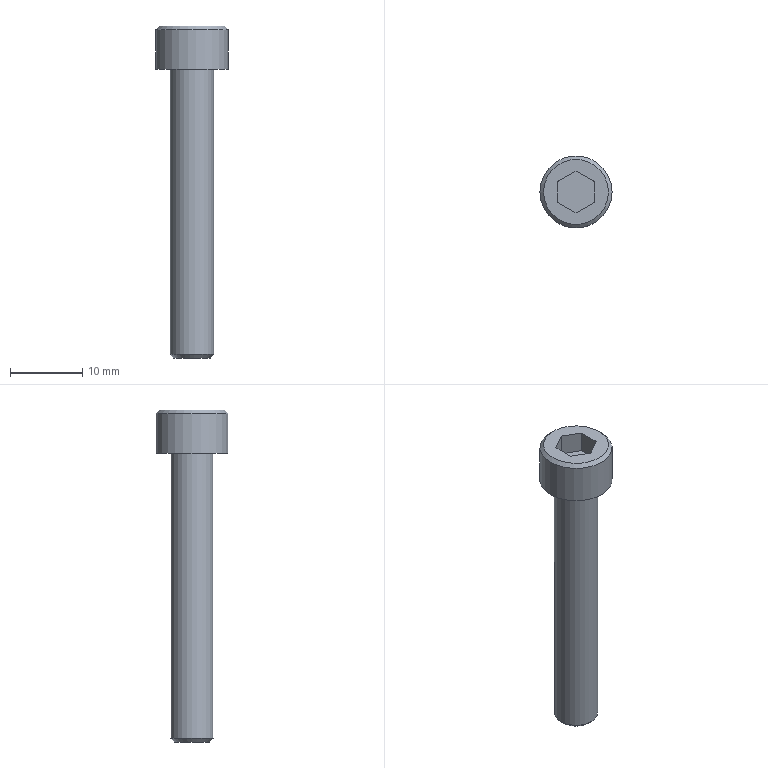Part | NX | features M6.00-50.00 2 | 1 solid | 14 faces | box 10 x 10 x 46 mm | volume 1531 mm3 | plane 10 | cylinder 2 | cone 2 | commonest cylinder face diameters 6 x1 10 x1
STEP:
#1=CARTESIAN_POINT('',(-39.5,190.75,-1.5));
#2=VERTEX_POINT('',#1);
#3=CARTESIAN_POINT('',(-44.,190.75,-1.5));
#4=DIRECTION('',(0.,0.,1.));
#5=DIRECTION('',(1.,0.,0.));
#6=AXIS2_PLACEMENT_3D('',#3,#4,#5);
#7=CIRCLE('',#6,4.5);
#8=EDGE_CURVE('',#2,#2,#7,.T.);
#9=ORIENTED_EDGE('',*,*,#8,.T.);
#10=EDGE_LOOP('',(#9));
#11=FACE_BOUND('',#10,.T.);
#12=CARTESIAN_POINT('',(-46.5,192.193,-1.5));
#13=VERTEX_POINT('',#12);
#14=CARTESIAN_POINT('',(-46.5,189.307,-1.5));
#15=VERTEX_POINT('',#14);
#16=CARTESIAN_POINT('',(-46.5,192.193,-1.5));
#17=DIRECTION('',(0.,-1.,0.));
#18=VECTOR('',#17,1000.);
#19=LINE('',#16,#18);
#20=EDGE_CURVE('',#13,#15,#19,.T.);
#21=ORIENTED_EDGE('',*,*,#20,.F.);
#22=CARTESIAN_POINT('',(-44.,193.637,-1.5));
#23=VERTEX_POINT('',#22);
#24=CARTESIAN_POINT('',(-44.,193.637,-1.5));
#25=DIRECTION('',(-0.866,-0.5,0.));
#26=VECTOR('',#25,1000.);
#27=LINE('',#24,#26);
#28=EDGE_CURVE('',#23,#13,#27,.T.);
#29=ORIENTED_EDGE('',*,*,#28,.F.);
#30=CARTESIAN_POINT('',(-41.5,192.193,-1.5));
#31=VERTEX_POINT('',#30);
#32=CARTESIAN_POINT('',(-41.5,192.193,-1.5));
#33=DIRECTION('',(-0.866,0.5,0.));
#34=VECTOR('',#33,1000.);
#35=LINE('',#32,#34);
#36=EDGE_CURVE('',#31,#23,#35,.T.);
#37=ORIENTED_EDGE('',*,*,#36,.F.);
#38=CARTESIAN_POINT('',(-41.5,189.307,-1.5));
#39=VERTEX_POINT('',#38);
#40=CARTESIAN_POINT('',(-41.5,189.307,-1.5));
#41=DIRECTION('',(0.,1.,0.));
#42=VECTOR('',#41,1000.);
#43=LINE('',#40,#42);
#44=EDGE_CURVE('',#39,#31,#43,.T.);
#45=ORIENTED_EDGE('',*,*,#44,.F.);
#46=CARTESIAN_POINT('',(-44.,187.863,-1.5));
#47=VERTEX_POINT('',#46);
#48=CARTESIAN_POINT('',(-44.,187.863,-1.5));
#49=DIRECTION('',(0.866,0.5,0.));
#50=VECTOR('',#49,1000.);
#51=LINE('',#48,#50);
#52=EDGE_CURVE('',#47,#39,#51,.T.);
#53=ORIENTED_EDGE('',*,*,#52,.F.);
#54=CARTESIAN_POINT('',(-46.5,189.307,-1.5));
#55=DIRECTION('',(0.866,-0.5,0.));
#56=VECTOR('',#55,1000.);
#57=LINE('',#54,#56);
#58=EDGE_CURVE('',#15,#47,#57,.T.);
#59=ORIENTED_EDGE('',*,*,#58,.F.);
#60=EDGE_LOOP('',(#21,#29,#37,#45,#53,#59));
#61=FACE_BOUND('',#60,.T.);
#62=CARTESIAN_POINT('',(-44.,190.75,-1.5));
#63=DIRECTION('',(0.,0.,1.));
#64=DIRECTION('',(1.,0.,0.));
#65=AXIS2_PLACEMENT_3D('',#62,#63,#64);
#66=PLANE('',#65);
#67=ADVANCED_FACE('',(#11,#61),#66,.T.);
#68=CARTESIAN_POINT('',(-41.,190.75,-7.5));
#69=VERTEX_POINT('',#68);
#70=CARTESIAN_POINT('',(-44.,190.75,-7.5));
#71=DIRECTION('',(0.,0.,-1.));
#72=DIRECTION('',(1.,0.,0.));
#73=AXIS2_PLACEMENT_3D('',#70,#71,#72);
#74=CIRCLE('',#73,3.);
#75=EDGE_CURVE('',#69,#69,#74,.T.);
#76=ORIENTED_EDGE('',*,*,#75,.F.);
#77=EDGE_LOOP('',(#76));
#78=FACE_BOUND('',#77,.T.);
#79=CARTESIAN_POINT('',(-39.,190.75,-7.5));
#80=VERTEX_POINT('',#79);
#81=CARTESIAN_POINT('',(-44.,190.75,-7.5));
#82=DIRECTION('',(0.,0.,1.));
#83=DIRECTION('',(1.,0.,0.));
#84=AXIS2_PLACEMENT_3D('',#81,#82,#83);
#85=CIRCLE('',#84,5.);
#86=EDGE_CURVE('',#80,#80,#85,.T.);
#87=ORIENTED_EDGE('',*,*,#86,.F.);
#88=EDGE_LOOP('',(#87));
#89=FACE_BOUND('',#88,.T.);
#90=CARTESIAN_POINT('',(-44.,190.75,-7.5));
#91=DIRECTION('',(0.,0.,-1.));
#92=DIRECTION('',(-1.,0.,0.));
#93=AXIS2_PLACEMENT_3D('',#90,#91,#92);
#94=PLANE('',#93);
#95=ADVANCED_FACE('',(#78,#89),#94,.T.);
#96=CARTESIAN_POINT('',(-39.,190.75,-2.));
#97=VERTEX_POINT('',#96);
#98=CARTESIAN_POINT('',(-44.,190.75,-2.));
#99=DIRECTION('',(0.,0.,1.));
#100=DIRECTION('',(1.,0.,0.));
#101=AXIS2_PLACEMENT_3D('',#98,#99,#100);
#102=CIRCLE('',#101,5.);
#103=EDGE_CURVE('',#97,#97,#102,.F.);
#104=ORIENTED_EDGE('',*,*,#103,.T.);
#105=EDGE_LOOP('',(#104));
#106=FACE_BOUND('',#105,.T.);
#107=ORIENTED_EDGE('',*,*,#86,.T.);
#108=EDGE_LOOP('',(#107));
#109=FACE_BOUND('',#108,.T.);
#110=CARTESIAN_POINT('',(-44.,190.75,-7.5));
#111=DIRECTION('',(0.,0.,1.));
#112=DIRECTION('',(1.,0.,0.));
#113=AXIS2_PLACEMENT_3D('',#110,#111,#112);
#114=CYLINDRICAL_SURFACE('',#113,5.);
#115=ADVANCED_FACE('',(#106,#109),#114,.T.);
#116=CARTESIAN_POINT('',(-46.5,190.75,-47.5));
#117=VERTEX_POINT('',#116);
#118=CARTESIAN_POINT('',(-44.,190.75,-47.5));
#119=DIRECTION('',(0.,0.,-1.));
#120=DIRECTION('',(-1.,0.,0.));
#121=AXIS2_PLACEMENT_3D('',#118,#119,#120);
#122=CIRCLE('',#121,2.5);
#123=EDGE_CURVE('',#117,#117,#122,.T.);
#124=ORIENTED_EDGE('',*,*,#123,.T.);
#125=EDGE_LOOP('',(#124));
#126=FACE_BOUND('',#125,.T.);
#127=CARTESIAN_POINT('',(-44.,190.75,-47.5));
#128=DIRECTION('',(0.,0.,-1.));
#129=DIRECTION('',(-1.,0.,0.));
#130=AXIS2_PLACEMENT_3D('',#127,#128,#129);
#131=PLANE('',#130);
#132=ADVANCED_FACE('',(#126),#131,.T.);
#133=CARTESIAN_POINT('',(-47.,190.75,-47.));
#134=VERTEX_POINT('',#133);
#135=CARTESIAN_POINT('',(-44.,190.75,-47.));
#136=DIRECTION('',(0.,0.,-1.));
#137=DIRECTION('',(-1.,0.,0.));
#138=AXIS2_PLACEMENT_3D('',#135,#136,#137);
#139=CIRCLE('',#138,3.);
#140=EDGE_CURVE('',#134,#134,#139,.F.);
#141=ORIENTED_EDGE('',*,*,#140,.T.);
#142=EDGE_LOOP('',(#141));
#143=FACE_BOUND('',#142,.T.);
#144=ORIENTED_EDGE('',*,*,#75,.T.);
#145=EDGE_LOOP('',(#144));
#146=FACE_BOUND('',#145,.T.);
#147=CARTESIAN_POINT('',(-44.,190.75,-7.5));
#148=DIRECTION('',(0.,0.,-1.));
#149=DIRECTION('',(1.,0.,0.));
#150=AXIS2_PLACEMENT_3D('',#147,#148,#149);
#151=CYLINDRICAL_SURFACE('',#150,3.);
#152=ADVANCED_FACE('',(#143,#146),#151,.T.);
#153=ORIENTED_EDGE('',*,*,#58,.T.);
#154=CARTESIAN_POINT('',(-44.,187.863,-4.5));
#155=VERTEX_POINT('',#154);
#156=CARTESIAN_POINT('',(-44.,187.863,-4.5));
#157=DIRECTION('',(0.,0.,1.));
#158=VECTOR('',#157,1000.);
#159=LINE('',#156,#158);
#160=EDGE_CURVE('',#47,#155,#159,.F.);
#161=ORIENTED_EDGE('',*,*,#160,.T.);
#162=CARTESIAN_POINT('',(-46.5,189.307,-4.5));
#163=VERTEX_POINT('',#162);
#164=CARTESIAN_POINT('',(-46.5,189.307,-4.5));
#165=DIRECTION('',(0.866,-0.5,0.));
#166=VECTOR('',#165,1000.);
#167=LINE('',#164,#166);
#168=EDGE_CURVE('',#155,#163,#167,.F.);
#169=ORIENTED_EDGE('',*,*,#168,.T.);
#170=CARTESIAN_POINT('',(-46.5,189.307,-4.5));
#171=DIRECTION('',(0.,0.,1.));
#172=VECTOR('',#171,1000.);
#173=LINE('',#170,#172);
#174=EDGE_CURVE('',#15,#163,#173,.F.);
#175=ORIENTED_EDGE('',*,*,#174,.F.);
#176=EDGE_LOOP('',(#153,#161,#169,#175));
#177=FACE_BOUND('',#176,.T.);
#178=CARTESIAN_POINT('',(-45.25,188.585,-3.));
#179=DIRECTION('',(-0.5,-0.866,0.));
#180=DIRECTION('',(0.866,-0.5,0.));
#181=AXIS2_PLACEMENT_3D('',#178,#179,#180);
#182=PLANE('',#181);
#183=ADVANCED_FACE('',(#177),#182,.F.);
#184=ORIENTED_EDGE('',*,*,#20,.T.);
#185=ORIENTED_EDGE('',*,*,#174,.T.);
#186=CARTESIAN_POINT('',(-46.5,192.193,-4.5));
#187=VERTEX_POINT('',#186);
#188=CARTESIAN_POINT('',(-46.5,192.193,-4.5));
#189=DIRECTION('',(0.,-1.,0.));
#190=VECTOR('',#189,1000.);
#191=LINE('',#188,#190);
#192=EDGE_CURVE('',#163,#187,#191,.F.);
#193=ORIENTED_EDGE('',*,*,#192,.T.);
#194=CARTESIAN_POINT('',(-46.5,192.193,-4.5));
#195=DIRECTION('',(0.,0.,1.));
#196=VECTOR('',#195,1000.);
#197=LINE('',#194,#196);
#198=EDGE_CURVE('',#13,#187,#197,.F.);
#199=ORIENTED_EDGE('',*,*,#198,.F.);
#200=EDGE_LOOP('',(#184,#185,#193,#199));
#201=FACE_BOUND('',#200,.T.);
#202=CARTESIAN_POINT('',(-46.5,190.75,-3.));
#203=DIRECTION('',(-1.,0.,0.));
#204=DIRECTION('',(0.,0.,1.));
#205=AXIS2_PLACEMENT_3D('',#202,#203,#204);
#206=PLANE('',#205);
#207=ADVANCED_FACE('',(#201),#206,.F.);
#208=ORIENTED_EDGE('',*,*,#28,.T.);
#209=ORIENTED_EDGE('',*,*,#198,.T.);
#210=CARTESIAN_POINT('',(-44.,193.637,-4.5));
#211=VERTEX_POINT('',#210);
#212=CARTESIAN_POINT('',(-44.,193.637,-4.5));
#213=DIRECTION('',(-0.866,-0.5,0.));
#214=VECTOR('',#213,1000.);
#215=LINE('',#212,#214);
#216=EDGE_CURVE('',#187,#211,#215,.F.);
#217=ORIENTED_EDGE('',*,*,#216,.T.);
#218=CARTESIAN_POINT('',(-44.,193.637,-4.5));
#219=DIRECTION('',(0.,0.,1.));
#220=VECTOR('',#219,1000.);
#221=LINE('',#218,#220);
#222=EDGE_CURVE('',#23,#211,#221,.F.);
#223=ORIENTED_EDGE('',*,*,#222,.F.);
#224=EDGE_LOOP('',(#208,#209,#217,#223));
#225=FACE_BOUND('',#224,.T.);
#226=CARTESIAN_POINT('',(-45.25,192.915,-3.));
#227=DIRECTION('',(-0.5,0.866,0.));
#228=DIRECTION('',(-0.866,-0.5,0.));
#229=AXIS2_PLACEMENT_3D('',#226,#227,#228);
#230=PLANE('',#229);
#231=ADVANCED_FACE('',(#225),#230,.F.);
#232=ORIENTED_EDGE('',*,*,#36,.T.);
#233=ORIENTED_EDGE('',*,*,#222,.T.);
#234=CARTESIAN_POINT('',(-41.5,192.193,-4.5));
#235=VERTEX_POINT('',#234);
#236=CARTESIAN_POINT('',(-41.5,192.193,-4.5));
#237=DIRECTION('',(-0.866,0.5,0.));
#238=VECTOR('',#237,1000.);
#239=LINE('',#236,#238);
#240=EDGE_CURVE('',#211,#235,#239,.F.);
#241=ORIENTED_EDGE('',*,*,#240,.T.);
#242=CARTESIAN_POINT('',(-41.5,192.193,-4.5));
#243=DIRECTION('',(0.,0.,1.));
#244=VECTOR('',#243,1000.);
#245=LINE('',#242,#244);
#246=EDGE_CURVE('',#31,#235,#245,.F.);
#247=ORIENTED_EDGE('',*,*,#246,.F.);
#248=EDGE_LOOP('',(#232,#233,#241,#247));
#249=FACE_BOUND('',#248,.T.);
#250=CARTESIAN_POINT('',(-42.75,192.915,-3.));
#251=DIRECTION('',(0.5,0.866,0.));
#252=DIRECTION('',(-0.866,0.5,0.));
#253=AXIS2_PLACEMENT_3D('',#250,#251,#252);
#254=PLANE('',#253);
#255=ADVANCED_FACE('',(#249),#254,.F.);
#256=ORIENTED_EDGE('',*,*,#44,.T.);
#257=ORIENTED_EDGE('',*,*,#246,.T.);
#258=CARTESIAN_POINT('',(-41.5,189.307,-4.5));
#259=VERTEX_POINT('',#258);
#260=CARTESIAN_POINT('',(-41.5,189.307,-4.5));
#261=DIRECTION('',(0.,1.,0.));
#262=VECTOR('',#261,1000.);
#263=LINE('',#260,#262);
#264=EDGE_CURVE('',#235,#259,#263,.F.);
#265=ORIENTED_EDGE('',*,*,#264,.T.);
#266=CARTESIAN_POINT('',(-41.5,189.307,-4.5));
#267=DIRECTION('',(0.,0.,1.));
#268=VECTOR('',#267,1000.);
#269=LINE('',#266,#268);
#270=EDGE_CURVE('',#39,#259,#269,.F.);
#271=ORIENTED_EDGE('',*,*,#270,.F.);
#272=EDGE_LOOP('',(#256,#257,#265,#271));
#273=FACE_BOUND('',#272,.T.);
#274=CARTESIAN_POINT('',(-41.5,190.75,-3.));
#275=DIRECTION('',(1.,0.,0.));
#276=DIRECTION('',(0.,0.,-1.));
#277=AXIS2_PLACEMENT_3D('',#274,#275,#276);
#278=PLANE('',#277);
#279=ADVANCED_FACE('',(#273),#278,.F.);
#280=ORIENTED_EDGE('',*,*,#52,.T.);
#281=ORIENTED_EDGE('',*,*,#270,.T.);
#282=CARTESIAN_POINT('',(-44.,187.863,-4.5));
#283=DIRECTION('',(0.866,0.5,0.));
#284=VECTOR('',#283,1000.);
#285=LINE('',#282,#284);
#286=EDGE_CURVE('',#259,#155,#285,.F.);
#287=ORIENTED_EDGE('',*,*,#286,.T.);
#288=ORIENTED_EDGE('',*,*,#160,.F.);
#289=EDGE_LOOP('',(#280,#281,#287,#288));
#290=FACE_BOUND('',#289,.T.);
#291=CARTESIAN_POINT('',(-42.75,188.585,-3.));
#292=DIRECTION('',(0.5,-0.866,0.));
#293=DIRECTION('',(0.866,0.5,0.));
#294=AXIS2_PLACEMENT_3D('',#291,#292,#293);
#295=PLANE('',#294);
#296=ADVANCED_FACE('',(#290),#295,.F.);
#297=ORIENTED_EDGE('',*,*,#286,.F.);
#298=ORIENTED_EDGE('',*,*,#264,.F.);
#299=ORIENTED_EDGE('',*,*,#240,.F.);
#300=ORIENTED_EDGE('',*,*,#216,.F.);
#301=ORIENTED_EDGE('',*,*,#192,.F.);
#302=ORIENTED_EDGE('',*,*,#168,.F.);
#303=EDGE_LOOP('',(#297,#298,#299,#300,#301,#302));
#304=FACE_BOUND('',#303,.T.);
#305=CARTESIAN_POINT('',(-44.,190.75,-4.5));
#306=DIRECTION('',(0.,0.,-1.));
#307=DIRECTION('',(-1.,0.,0.));
#308=AXIS2_PLACEMENT_3D('',#305,#306,#307);
#309=PLANE('',#308);
#310=ADVANCED_FACE('',(#304),#309,.F.);
#311=ORIENTED_EDGE('',*,*,#123,.F.);
#312=EDGE_LOOP('',(#311));
#313=FACE_BOUND('',#312,.T.);
#314=ORIENTED_EDGE('',*,*,#140,.F.);
#315=EDGE_LOOP('',(#314));
#316=FACE_BOUND('',#315,.T.);
#317=CARTESIAN_POINT('',(-44.,190.75,-47.));
#318=DIRECTION('',(0.,0.,1.));
#319=DIRECTION('',(1.,0.,0.));
#320=AXIS2_PLACEMENT_3D('',#317,#318,#319);
#321=CONICAL_SURFACE('',#320,3.,0.7854);
#322=ADVANCED_FACE('',(#313,#316),#321,.T.);
#323=ORIENTED_EDGE('',*,*,#8,.F.);
#324=EDGE_LOOP('',(#323));
#325=FACE_BOUND('',#324,.T.);
#326=ORIENTED_EDGE('',*,*,#103,.F.);
#327=EDGE_LOOP('',(#326));
#328=FACE_BOUND('',#327,.T.);
#329=CARTESIAN_POINT('',(-44.,190.75,-2.));
#330=DIRECTION('',(0.,0.,-1.));
#331=DIRECTION('',(-1.,0.,0.));
#332=AXIS2_PLACEMENT_3D('',#329,#330,#331);
#333=CONICAL_SURFACE('',#332,5.,0.7854);
#334=ADVANCED_FACE('',(#325,#328),#333,.T.);
#335=CLOSED_SHELL('',(#67,#95,#115,#132,#152,#183,#207,#231,#255,#279,#296,#310,#322,#334));
#336=MANIFOLD_SOLID_BREP('',#335);
#337=(LENGTH_UNIT()NAMED_UNIT(*)SI_UNIT(.MILLI.,.METRE.));
#338=UNCERTAINTY_MEASURE_WITH_UNIT(LENGTH_MEASURE(0.00001),#337,'','');
#339=(NAMED_UNIT(*)PLANE_ANGLE_UNIT()SI_UNIT($,.RADIAN.));
#340=(NAMED_UNIT(*)SI_UNIT($,.STERADIAN.)SOLID_ANGLE_UNIT());
#341=(GEOMETRIC_REPRESENTATION_CONTEXT(3)GLOBAL_UNCERTAINTY_ASSIGNED_CONTEXT((#338))GLOBAL_UNIT_ASSIGNED_CONTEXT((#337,#339,#340))REPRESENTATION_CONTEXT('',''));
#342=ADVANCED_BREP_SHAPE_REPRESENTATION('',(#336),#341);